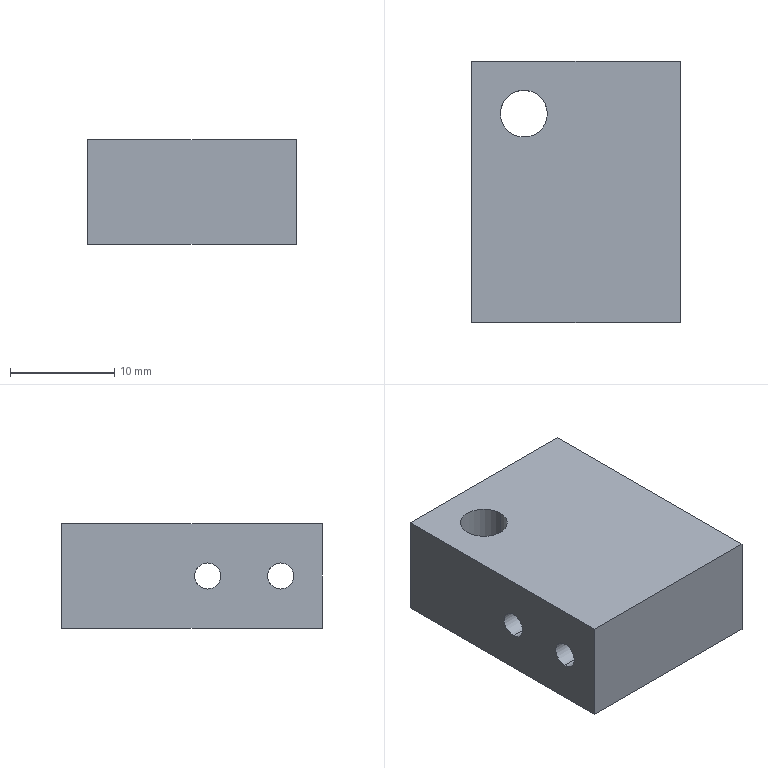Part | STEP file | 10-27 air distribution block | 1 solid | 19 faces | box 20 x 25 x 10 mm | volume 4387 mm3 | cylinder 10 | plane 6 | cone 3 | commonest cylinder face diameters 2.5 x6 4.2 x2 4.5 x2
STEP:
#1=CARTESIAN_POINT('',(0.3125,-1.5,3.75));
#2=VERTEX_POINT('',#1);
#3=CARTESIAN_POINT('',(0.3125,-1.5,6.25));
#4=VERTEX_POINT('',#3);
#5=CARTESIAN_POINT('',(0.3125,-1.5,3.75));
#6=CARTESIAN_POINT('',(0.3125,-1.415,3.75));
#7=CARTESIAN_POINT('',(0.3061,-1.332,3.759));
#8=CARTESIAN_POINT('',(0.2824,-1.17,3.792));
#9=CARTESIAN_POINT('',(0.2649,-1.09,3.816));
#10=CARTESIAN_POINT('',(0.2029,-0.8652,3.911));
#11=CARTESIAN_POINT('',(0.148,-0.7304,4.002));
#12=CARTESIAN_POINT('',(0.04358,-0.505,4.227));
#13=CARTESIAN_POINT('',(-0.006727,-0.4127,4.362));
#14=CARTESIAN_POINT('',(-0.06054,-0.3172,4.588));
#15=CARTESIAN_POINT('',(-0.07523,-0.292,4.668));
#16=CARTESIAN_POINT('',(-0.09477,-0.2587,4.831));
#17=CARTESIAN_POINT('',(-0.09991,-0.2502,4.914));
#18=CARTESIAN_POINT('',(-0.1002,-0.2497,5.166));
#19=CARTESIAN_POINT('',(-0.07907,-0.2843,5.334));
#20=CARTESIAN_POINT('',(-0.007079,-0.412,5.637));
#21=CARTESIAN_POINT('',(0.04343,-0.5047,5.773));
#22=CARTESIAN_POINT('',(0.1479,-0.7302,5.998));
#23=CARTESIAN_POINT('',(0.2027,-0.865,6.089));
#24=CARTESIAN_POINT('',(0.2646,-1.089,6.183));
#25=CARTESIAN_POINT('',(0.2822,-1.169,6.208));
#26=CARTESIAN_POINT('',(0.3061,-1.332,6.241));
#27=CARTESIAN_POINT('',(0.3125,-1.415,6.25));
#28=CARTESIAN_POINT('',(0.3125,-1.5,6.25));
#29=B_SPLINE_CURVE_WITH_KNOTS('',3,(#5,#6,#7,#8,#9,#10,#11,#12,#13,#14,#15,#16,#17,#18,#19,#20,#21,#22,#23,#24,#25,#26,#27,#28),.UNSPECIFIED.,.F.,.F.,(4,2,2,2,2,2,2,2,2,2,2,4),(0.,0.0002504,0.0005009,0.001002,0.001503,0.001753,0.002003,0.002504,0.003005,0.003506,0.003756,0.004007),.UNSPECIFIED.);
#30=EDGE_CURVE('',#2,#4,#29,.T.);
#31=ORIENTED_EDGE('',*,*,#30,.F.);
#32=CARTESIAN_POINT('',(0.3125,-1.5,6.25));
#33=CARTESIAN_POINT('',(0.3125,-1.67,6.25));
#34=CARTESIAN_POINT('',(0.2855,-1.836,6.215));
#35=CARTESIAN_POINT('',(0.2027,-2.135,6.089));
#36=CARTESIAN_POINT('',(0.1479,-2.27,5.998));
#37=CARTESIAN_POINT('',(0.04322,-2.496,5.772));
#38=CARTESIAN_POINT('',(-0.006762,-2.587,5.638));
#39=CARTESIAN_POINT('',(-0.06081,-2.683,5.411));
#40=CARTESIAN_POINT('',(-0.07535,-2.708,5.331));
#41=CARTESIAN_POINT('',(-0.09479,-2.741,5.169));
#42=CARTESIAN_POINT('',(-0.09996,-2.75,5.086));
#43=CARTESIAN_POINT('',(-0.1,-2.75,4.916));
#44=CARTESIAN_POINT('',(-0.09495,-2.742,4.833));
#45=CARTESIAN_POINT('',(-0.07549,-2.708,4.67));
#46=CARTESIAN_POINT('',(-0.06088,-2.683,4.589));
#47=CARTESIAN_POINT('',(-0.006947,-2.588,4.363));
#48=CARTESIAN_POINT('',(0.04358,-2.495,4.227));
#49=CARTESIAN_POINT('',(0.1483,-2.269,4.002));
#50=CARTESIAN_POINT('',(0.2028,-2.135,3.911));
#51=CARTESIAN_POINT('',(0.2649,-1.91,3.816));
#52=CARTESIAN_POINT('',(0.2825,-1.83,3.792));
#53=CARTESIAN_POINT('',(0.3061,-1.668,3.759));
#54=CARTESIAN_POINT('',(0.3125,-1.585,3.75));
#55=CARTESIAN_POINT('',(0.3125,-1.5,3.75));
#56=B_SPLINE_CURVE_WITH_KNOTS('',3,(#32,#33,#34,#35,#36,#37,#38,#39,#40,#41,#42,#43,#44,#45,#46,#47,#48,#49,#50,#51,#52,#53,#54,#55),.UNSPECIFIED.,.F.,.F.,(4,2,2,2,2,2,2,2,2,2,2,4),(0.004007,0.004507,0.005007,0.005507,0.005757,0.006007,0.006256,0.006506,0.007006,0.007506,0.007756,0.008006),.UNSPECIFIED.);
#57=EDGE_CURVE('',#4,#2,#56,.T.);
#58=ORIENTED_EDGE('',*,*,#57,.F.);
#59=EDGE_LOOP('',(#31,#58));
#60=FACE_BOUND('',#59,.T.);
#61=CARTESIAN_POINT('',(2.,-7.5,2.9));
#62=VERTEX_POINT('',#61);
#63=CARTESIAN_POINT('',(0.0385,-7.5,4.25));
#64=VERTEX_POINT('',#63);
#65=CARTESIAN_POINT('',(2.,-7.5,5.));
#66=DIRECTION('',(0.,1.,0.));
#67=DIRECTION('',(0.,0.,1.));
#68=AXIS2_PLACEMENT_3D('',#65,#66,#67);
#69=CIRCLE('',#68,2.1);
#70=EDGE_CURVE('',#62,#64,#69,.T.);
#71=ORIENTED_EDGE('',*,*,#70,.F.);
#72=CARTESIAN_POINT('',(2.,12.5,2.9));
#73=VERTEX_POINT('',#72);
#74=CARTESIAN_POINT('',(2.,12.5,2.9));
#75=DIRECTION('',(0.,1.,0.));
#76=VECTOR('',#75,1000.);
#77=LINE('',#74,#76);
#78=EDGE_CURVE('',#62,#73,#77,.T.);
#79=ORIENTED_EDGE('',*,*,#78,.T.);
#80=CARTESIAN_POINT('',(2.,12.5,7.1));
#81=VERTEX_POINT('',#80);
#82=CARTESIAN_POINT('',(2.,12.5,5.));
#83=DIRECTION('',(0.,1.,0.));
#84=DIRECTION('',(0.,0.,1.));
#85=AXIS2_PLACEMENT_3D('',#82,#83,#84);
#86=CIRCLE('',#85,2.1);
#87=EDGE_CURVE('',#73,#81,#86,.T.);
#88=ORIENTED_EDGE('',*,*,#87,.T.);
#89=CARTESIAN_POINT('',(2.,-7.5,7.1));
#90=VERTEX_POINT('',#89);
#91=CARTESIAN_POINT('',(2.,12.5,7.1));
#92=DIRECTION('',(0.,1.,0.));
#93=VECTOR('',#92,1000.);
#94=LINE('',#91,#93);
#95=EDGE_CURVE('',#90,#81,#94,.T.);
#96=ORIENTED_EDGE('',*,*,#95,.F.);
#97=CARTESIAN_POINT('',(0.0385,-7.5,5.75));
#98=VERTEX_POINT('',#97);
#99=CARTESIAN_POINT('',(2.,-7.5,5.));
#100=DIRECTION('',(0.,1.,0.));
#101=DIRECTION('',(0.,0.,1.));
#102=AXIS2_PLACEMENT_3D('',#99,#100,#101);
#103=CIRCLE('',#102,2.1);
#104=EDGE_CURVE('',#98,#90,#103,.T.);
#105=ORIENTED_EDGE('',*,*,#104,.F.);
#106=CARTESIAN_POINT('',(0.0385,-7.5,4.25));
#107=CARTESIAN_POINT('',(-0.001759,-7.421,4.355));
#108=CARTESIAN_POINT('',(-0.03659,-7.359,4.471));
#109=CARTESIAN_POINT('',(-0.0864,-7.272,4.728));
#110=CARTESIAN_POINT('',(-0.09994,-7.25,4.861));
#111=CARTESIAN_POINT('',(-0.1001,-7.25,5.275));
#112=CARTESIAN_POINT('',(-0.04206,-7.342,5.539));
#113=CARTESIAN_POINT('',(0.0385,-7.5,5.75));
#114=B_SPLINE_CURVE_WITH_KNOTS('',3,(#106,#107,#108,#109,#110,#111,#112,#113),.UNSPECIFIED.,.F.,.F.,(4,2,2,4),(0.,0.0004077,0.0008154,0.001631),.UNSPECIFIED.);
#115=EDGE_CURVE('',#64,#98,#114,.T.);
#116=ORIENTED_EDGE('',*,*,#115,.F.);
#117=EDGE_LOOP('',(#71,#79,#88,#96,#105,#116));
#118=FACE_OUTER_BOUND('',#117,.T.);
#119=CARTESIAN_POINT('',(2.,12.5,5.));
#120=DIRECTION('',(0.,1.,0.));
#121=DIRECTION('',(0.,0.,1.));
#122=AXIS2_PLACEMENT_3D('',#119,#120,#121);
#123=CYLINDRICAL_SURFACE('',#122,2.1);
#124=ADVANCED_FACE('',(#60,#118),#123,.F.);
#125=CARTESIAN_POINT('',(2.,-8.059,6.17));
#126=VERTEX_POINT('',#125);
#127=CARTESIAN_POINT('',(3.962,-7.5,5.75));
#128=VERTEX_POINT('',#127);
#129=CARTESIAN_POINT('',(2.,-8.059,6.17));
#130=CARTESIAN_POINT('',(2.176,-8.059,6.17));
#131=CARTESIAN_POINT('',(2.354,-8.038,6.162));
#132=CARTESIAN_POINT('',(2.697,-7.969,6.132));
#133=CARTESIAN_POINT('',(2.865,-7.921,6.11));
#134=CARTESIAN_POINT('',(3.195,-7.811,6.045));
#135=CARTESIAN_POINT('',(3.355,-7.751,6.004));
#136=CARTESIAN_POINT('',(3.666,-7.627,5.898));
#137=CARTESIAN_POINT('',(3.818,-7.563,5.833));
#138=CARTESIAN_POINT('',(3.962,-7.5,5.75));
#139=B_SPLINE_CURVE_WITH_KNOTS('',3,(#129,#130,#131,#132,#133,#134,#135,#136,#137,#138),.UNSPECIFIED.,.F.,.F.,(4,2,2,2,4),(0.002488,0.003016,0.003543,0.00407,0.004597),.UNSPECIFIED.);
#140=EDGE_CURVE('',#126,#128,#139,.T.);
#141=ORIENTED_EDGE('',*,*,#140,.F.);
#142=CARTESIAN_POINT('',(2.,-7.5,7.1));
#143=DIRECTION('',(0.,0.515,0.8572));
#144=VECTOR('',#143,1000.);
#145=LINE('',#142,#144);
#146=EDGE_CURVE('',#126,#90,#145,.T.);
#147=ORIENTED_EDGE('',*,*,#146,.T.);
#148=CARTESIAN_POINT('',(2.,-7.5,5.));
#149=DIRECTION('',(0.,1.,0.));
#150=DIRECTION('',(0.,0.,1.));
#151=AXIS2_PLACEMENT_3D('',#148,#149,#150);
#152=CIRCLE('',#151,2.1);
#153=EDGE_CURVE('',#90,#128,#152,.T.);
#154=ORIENTED_EDGE('',*,*,#153,.T.);
#155=EDGE_LOOP('',(#141,#147,#154));
#156=FACE_OUTER_BOUND('',#155,.T.);
#157=CARTESIAN_POINT('',(2.,-7.5,5.));
#158=DIRECTION('',(0.,1.,0.));
#159=DIRECTION('',(0.,0.,1.));
#160=AXIS2_PLACEMENT_3D('',#157,#158,#159);
#161=CONICAL_SURFACE('',#160,2.1,1.03);
#162=ADVANCED_FACE('',(#156),#161,.F.);
#163=CARTESIAN_POINT('',(-10.,-8.5,6.25));
#164=VERTEX_POINT('',#163);
#165=CARTESIAN_POINT('',(-10.,-8.5,3.75));
#166=VERTEX_POINT('',#165);
#167=CARTESIAN_POINT('',(-10.,-8.5,5.));
#168=DIRECTION('',(1.,0.,0.));
#169=DIRECTION('',(0.,0.,-1.));
#170=AXIS2_PLACEMENT_3D('',#167,#168,#169);
#171=CIRCLE('',#170,1.25);
#172=EDGE_CURVE('',#164,#166,#171,.T.);
#173=ORIENTED_EDGE('',*,*,#172,.F.);
#174=CARTESIAN_POINT('',(10.,-8.5,6.25));
#175=VERTEX_POINT('',#174);
#176=CARTESIAN_POINT('',(10.,-8.5,6.25));
#177=DIRECTION('',(1.,0.,0.));
#178=VECTOR('',#177,1000.);
#179=LINE('',#176,#178);
#180=EDGE_CURVE('',#164,#175,#179,.T.);
#181=ORIENTED_EDGE('',*,*,#180,.T.);
#182=CARTESIAN_POINT('',(10.,-8.5,3.75));
#183=VERTEX_POINT('',#182);
#184=CARTESIAN_POINT('',(10.,-8.5,5.));
#185=DIRECTION('',(1.,0.,0.));
#186=DIRECTION('',(0.,0.,-1.));
#187=AXIS2_PLACEMENT_3D('',#184,#185,#186);
#188=CIRCLE('',#187,1.25);
#189=EDGE_CURVE('',#175,#183,#188,.T.);
#190=ORIENTED_EDGE('',*,*,#189,.T.);
#191=CARTESIAN_POINT('',(10.,-8.5,3.75));
#192=DIRECTION('',(1.,0.,0.));
#193=VECTOR('',#192,1000.);
#194=LINE('',#191,#193);
#195=EDGE_CURVE('',#166,#183,#194,.T.);
#196=ORIENTED_EDGE('',*,*,#195,.F.);
#197=EDGE_LOOP('',(#173,#181,#190,#196));
#198=FACE_OUTER_BOUND('',#197,.T.);
#199=CARTESIAN_POINT('',(10.,-8.5,5.));
#200=DIRECTION('',(1.,0.,0.));
#201=DIRECTION('',(0.,0.,-1.));
#202=AXIS2_PLACEMENT_3D('',#199,#200,#201);
#203=CYLINDRICAL_SURFACE('',#202,1.25);
#204=ADVANCED_FACE('',(#198),#203,.F.);
#205=CARTESIAN_POINT('',(3.687,-1.5,3.75));
#206=VERTEX_POINT('',#205);
#207=CARTESIAN_POINT('',(3.687,-1.5,6.25));
#208=VERTEX_POINT('',#207);
#209=CARTESIAN_POINT('',(3.687,-1.5,3.75));
#210=CARTESIAN_POINT('',(3.687,-1.585,3.75));
#211=CARTESIAN_POINT('',(3.694,-1.668,3.759));
#212=CARTESIAN_POINT('',(3.718,-1.83,3.792));
#213=CARTESIAN_POINT('',(3.735,-1.91,3.816));
#214=CARTESIAN_POINT('',(3.797,-2.135,3.911));
#215=CARTESIAN_POINT('',(3.852,-2.27,4.002));
#216=CARTESIAN_POINT('',(3.956,-2.495,4.227));
#217=CARTESIAN_POINT('',(4.007,-2.587,4.362));
#218=CARTESIAN_POINT('',(4.061,-2.683,4.588));
#219=CARTESIAN_POINT('',(4.075,-2.708,4.668));
#220=CARTESIAN_POINT('',(4.095,-2.741,4.831));
#221=CARTESIAN_POINT('',(4.1,-2.75,4.914));
#222=CARTESIAN_POINT('',(4.1,-2.75,5.166));
#223=CARTESIAN_POINT('',(4.079,-2.716,5.334));
#224=CARTESIAN_POINT('',(4.007,-2.588,5.637));
#225=CARTESIAN_POINT('',(3.957,-2.495,5.773));
#226=CARTESIAN_POINT('',(3.852,-2.27,5.998));
#227=CARTESIAN_POINT('',(3.797,-2.135,6.089));
#228=CARTESIAN_POINT('',(3.735,-1.911,6.183));
#229=CARTESIAN_POINT('',(3.718,-1.831,6.208));
#230=CARTESIAN_POINT('',(3.694,-1.668,6.241));
#231=CARTESIAN_POINT('',(3.687,-1.585,6.25));
#232=CARTESIAN_POINT('',(3.687,-1.5,6.25));
#233=B_SPLINE_CURVE_WITH_KNOTS('',3,(#209,#210,#211,#212,#213,#214,#215,#216,#217,#218,#219,#220,#221,#222,#223,#224,#225,#226,#227,#228,#229,#230,#231,#232),.UNSPECIFIED.,.F.,.F.,(4,2,2,2,2,2,2,2,2,2,2,4),(0.,0.0002504,0.0005009,0.001002,0.001503,0.001753,0.002003,0.002504,0.003005,0.003506,0.003756,0.004007),.UNSPECIFIED.);
#234=EDGE_CURVE('',#206,#208,#233,.T.);
#235=ORIENTED_EDGE('',*,*,#234,.T.);
#236=CARTESIAN_POINT('',(10.,-1.5,6.25));
#237=VERTEX_POINT('',#236);
#238=CARTESIAN_POINT('',(10.,-1.5,6.25));
#239=DIRECTION('',(1.,0.,0.));
#240=VECTOR('',#239,1000.);
#241=LINE('',#238,#240);
#242=EDGE_CURVE('',#208,#237,#241,.T.);
#243=ORIENTED_EDGE('',*,*,#242,.T.);
#244=CARTESIAN_POINT('',(10.,-1.5,3.75));
#245=VERTEX_POINT('',#244);
#246=CARTESIAN_POINT('',(10.,-1.5,5.));
#247=DIRECTION('',(1.,0.,0.));
#248=DIRECTION('',(0.,0.,-1.));
#249=AXIS2_PLACEMENT_3D('',#246,#247,#248);
#250=CIRCLE('',#249,1.25);
#251=EDGE_CURVE('',#237,#245,#250,.T.);
#252=ORIENTED_EDGE('',*,*,#251,.T.);
#253=CARTESIAN_POINT('',(10.,-1.5,3.75));
#254=DIRECTION('',(1.,0.,0.));
#255=VECTOR('',#254,1000.);
#256=LINE('',#253,#255);
#257=EDGE_CURVE('',#206,#245,#256,.T.);
#258=ORIENTED_EDGE('',*,*,#257,.F.);
#259=EDGE_LOOP('',(#235,#243,#252,#258));
#260=FACE_OUTER_BOUND('',#259,.T.);
#261=CARTESIAN_POINT('',(10.,-1.5,5.));
#262=DIRECTION('',(1.,0.,0.));
#263=DIRECTION('',(0.,0.,-1.));
#264=AXIS2_PLACEMENT_3D('',#261,#262,#263);
#265=CYLINDRICAL_SURFACE('',#264,1.25);
#266=ADVANCED_FACE('',(#260),#265,.F.);
#267=CARTESIAN_POINT('',(-7.25,7.5,0.));
#268=VERTEX_POINT('',#267);
#269=CARTESIAN_POINT('',(-2.75,7.5,0.));
#270=VERTEX_POINT('',#269);
#271=CARTESIAN_POINT('',(-5.,7.5,0.));
#272=DIRECTION('',(0.,0.,1.));
#273=DIRECTION('',(1.,0.,0.));
#274=AXIS2_PLACEMENT_3D('',#271,#272,#273);
#275=CIRCLE('',#274,2.25);
#276=EDGE_CURVE('',#268,#270,#275,.T.);
#277=ORIENTED_EDGE('',*,*,#276,.F.);
#278=CARTESIAN_POINT('',(-7.25,7.5,10.));
#279=VERTEX_POINT('',#278);
#280=CARTESIAN_POINT('',(-7.25,7.5,0.));
#281=DIRECTION('',(0.,0.,1.));
#282=VECTOR('',#281,1000.);
#283=LINE('',#280,#282);
#284=EDGE_CURVE('',#268,#279,#283,.T.);
#285=ORIENTED_EDGE('',*,*,#284,.T.);
#286=CARTESIAN_POINT('',(-2.75,7.5,10.));
#287=VERTEX_POINT('',#286);
#288=CARTESIAN_POINT('',(-5.,7.5,10.));
#289=DIRECTION('',(0.,0.,1.));
#290=DIRECTION('',(1.,0.,0.));
#291=AXIS2_PLACEMENT_3D('',#288,#289,#290);
#292=CIRCLE('',#291,2.25);
#293=EDGE_CURVE('',#279,#287,#292,.T.);
#294=ORIENTED_EDGE('',*,*,#293,.T.);
#295=CARTESIAN_POINT('',(-2.75,7.5,0.));
#296=DIRECTION('',(0.,0.,1.));
#297=VECTOR('',#296,1000.);
#298=LINE('',#295,#297);
#299=EDGE_CURVE('',#270,#287,#298,.T.);
#300=ORIENTED_EDGE('',*,*,#299,.F.);
#301=EDGE_LOOP('',(#277,#285,#294,#300));
#302=FACE_OUTER_BOUND('',#301,.T.);
#303=CARTESIAN_POINT('',(-5.,7.5,0.));
#304=DIRECTION('',(0.,0.,1.));
#305=DIRECTION('',(1.,0.,0.));
#306=AXIS2_PLACEMENT_3D('',#303,#304,#305);
#307=CYLINDRICAL_SURFACE('',#306,2.25);
#308=ADVANCED_FACE('',(#302),#307,.F.);
#309=CARTESIAN_POINT('',(-10.,-1.5,6.25));
#310=VERTEX_POINT('',#309);
#311=CARTESIAN_POINT('',(-10.,-1.5,3.75));
#312=VERTEX_POINT('',#311);
#313=CARTESIAN_POINT('',(-10.,-1.5,5.));
#314=DIRECTION('',(1.,0.,0.));
#315=DIRECTION('',(0.,0.,-1.));
#316=AXIS2_PLACEMENT_3D('',#313,#314,#315);
#317=CIRCLE('',#316,1.25);
#318=EDGE_CURVE('',#310,#312,#317,.T.);
#319=ORIENTED_EDGE('',*,*,#318,.F.);
#320=CARTESIAN_POINT('',(10.,-1.5,6.25));
#321=DIRECTION('',(1.,0.,0.));
#322=VECTOR('',#321,1000.);
#323=LINE('',#320,#322);
#324=EDGE_CURVE('',#310,#4,#323,.T.);
#325=ORIENTED_EDGE('',*,*,#324,.T.);
#326=ORIENTED_EDGE('',*,*,#57,.T.);
#327=CARTESIAN_POINT('',(10.,-1.5,3.75));
#328=DIRECTION('',(1.,0.,0.));
#329=VECTOR('',#328,1000.);
#330=LINE('',#327,#329);
#331=EDGE_CURVE('',#312,#2,#330,.T.);
#332=ORIENTED_EDGE('',*,*,#331,.F.);
#333=EDGE_LOOP('',(#319,#325,#326,#332));
#334=FACE_OUTER_BOUND('',#333,.T.);
#335=CARTESIAN_POINT('',(10.,-1.5,5.));
#336=DIRECTION('',(1.,0.,0.));
#337=DIRECTION('',(0.,0.,-1.));
#338=AXIS2_PLACEMENT_3D('',#335,#336,#337);
#339=CYLINDRICAL_SURFACE('',#338,1.25);
#340=ADVANCED_FACE('',(#334),#339,.F.);
#341=ORIENTED_EDGE('',*,*,#324,.F.);
#342=CARTESIAN_POINT('',(-10.,-1.5,5.));
#343=DIRECTION('',(1.,0.,0.));
#344=DIRECTION('',(0.,0.,-1.));
#345=AXIS2_PLACEMENT_3D('',#342,#343,#344);
#346=CIRCLE('',#345,1.25);
#347=EDGE_CURVE('',#312,#310,#346,.T.);
#348=ORIENTED_EDGE('',*,*,#347,.F.);
#349=ORIENTED_EDGE('',*,*,#331,.T.);
#350=ORIENTED_EDGE('',*,*,#30,.T.);
#351=EDGE_LOOP('',(#341,#348,#349,#350));
#352=FACE_OUTER_BOUND('',#351,.T.);
#353=CARTESIAN_POINT('',(10.,-1.5,5.));
#354=DIRECTION('',(1.,0.,0.));
#355=DIRECTION('',(0.,0.,-1.));
#356=AXIS2_PLACEMENT_3D('',#353,#354,#355);
#357=CYLINDRICAL_SURFACE('',#356,1.25);
#358=ADVANCED_FACE('',(#352),#357,.F.);
#359=CARTESIAN_POINT('',(10.,-8.5,5.));
#360=DIRECTION('',(1.,0.,0.));
#361=DIRECTION('',(0.,0.,-1.));
#362=AXIS2_PLACEMENT_3D('',#359,#360,#361);
#363=CIRCLE('',#362,1.25);
#364=EDGE_CURVE('',#183,#175,#363,.T.);
#365=ORIENTED_EDGE('',*,*,#364,.F.);
#366=ORIENTED_EDGE('',*,*,#189,.F.);
#367=EDGE_LOOP('',(#365,#366));
#368=FACE_BOUND('',#367,.T.);
#369=CARTESIAN_POINT('',(10.,-1.5,5.));
#370=DIRECTION('',(1.,0.,0.));
#371=DIRECTION('',(0.,0.,-1.));
#372=AXIS2_PLACEMENT_3D('',#369,#370,#371);
#373=CIRCLE('',#372,1.25);
#374=EDGE_CURVE('',#245,#237,#373,.T.);
#375=ORIENTED_EDGE('',*,*,#374,.F.);
#376=ORIENTED_EDGE('',*,*,#251,.F.);
#377=EDGE_LOOP('',(#375,#376));
#378=FACE_BOUND('',#377,.T.);
#379=CARTESIAN_POINT('',(10.,-12.5,0.));
#380=VERTEX_POINT('',#379);
#381=CARTESIAN_POINT('',(10.,12.5,0.));
#382=VERTEX_POINT('',#381);
#383=CARTESIAN_POINT('',(10.,12.5,0.));
#384=DIRECTION('',(0.,1.,0.));
#385=VECTOR('',#384,1000.);
#386=LINE('',#383,#385);
#387=EDGE_CURVE('',#380,#382,#386,.T.);
#388=ORIENTED_EDGE('',*,*,#387,.T.);
#389=CARTESIAN_POINT('',(10.,12.5,10.));
#390=VERTEX_POINT('',#389);
#391=CARTESIAN_POINT('',(10.,12.5,10.));
#392=DIRECTION('',(0.,0.,-1.));
#393=VECTOR('',#392,1000.);
#394=LINE('',#391,#393);
#395=EDGE_CURVE('',#390,#382,#394,.T.);
#396=ORIENTED_EDGE('',*,*,#395,.F.);
#397=CARTESIAN_POINT('',(10.,-12.5,10.));
#398=VERTEX_POINT('',#397);
#399=CARTESIAN_POINT('',(10.,12.5,10.));
#400=DIRECTION('',(0.,1.,0.));
#401=VECTOR('',#400,1000.);
#402=LINE('',#399,#401);
#403=EDGE_CURVE('',#398,#390,#402,.T.);
#404=ORIENTED_EDGE('',*,*,#403,.F.);
#405=CARTESIAN_POINT('',(10.,-12.5,10.));
#406=DIRECTION('',(0.,0.,-1.));
#407=VECTOR('',#406,1000.);
#408=LINE('',#405,#407);
#409=EDGE_CURVE('',#398,#380,#408,.T.);
#410=ORIENTED_EDGE('',*,*,#409,.T.);
#411=EDGE_LOOP('',(#388,#396,#404,#410));
#412=FACE_OUTER_BOUND('',#411,.T.);
#413=CARTESIAN_POINT('',(10.,12.5,10.));
#414=DIRECTION('',(-1.,0.,0.));
#415=DIRECTION('',(0.,-1.,0.));
#416=AXIS2_PLACEMENT_3D('',#413,#414,#415);
#417=PLANE('',#416);
#418=ADVANCED_FACE('',(#368,#378,#412),#417,.F.);
#419=CARTESIAN_POINT('',(2.,12.5,5.));
#420=DIRECTION('',(0.,1.,0.));
#421=DIRECTION('',(0.,0.,1.));
#422=AXIS2_PLACEMENT_3D('',#419,#420,#421);
#423=CIRCLE('',#422,2.1);
#424=EDGE_CURVE('',#81,#73,#423,.T.);
#425=ORIENTED_EDGE('',*,*,#424,.F.);
#426=ORIENTED_EDGE('',*,*,#87,.F.);
#427=EDGE_LOOP('',(#425,#426));
#428=FACE_BOUND('',#427,.T.);
#429=CARTESIAN_POINT('',(-10.,12.5,0.));
#430=VERTEX_POINT('',#429);
#431=CARTESIAN_POINT('',(-10.,12.5,0.));
#432=DIRECTION('',(-1.,0.,0.));
#433=VECTOR('',#432,1000.);
#434=LINE('',#431,#433);
#435=EDGE_CURVE('',#382,#430,#434,.T.);
#436=ORIENTED_EDGE('',*,*,#435,.T.);
#437=CARTESIAN_POINT('',(-10.,12.5,10.));
#438=VERTEX_POINT('',#437);
#439=CARTESIAN_POINT('',(-10.,12.5,10.));
#440=DIRECTION('',(0.,0.,-1.));
#441=VECTOR('',#440,1000.);
#442=LINE('',#439,#441);
#443=EDGE_CURVE('',#438,#430,#442,.T.);
#444=ORIENTED_EDGE('',*,*,#443,.F.);
#445=CARTESIAN_POINT('',(-10.,12.5,10.));
#446=DIRECTION('',(-1.,0.,0.));
#447=VECTOR('',#446,1000.);
#448=LINE('',#445,#447);
#449=EDGE_CURVE('',#390,#438,#448,.T.);
#450=ORIENTED_EDGE('',*,*,#449,.F.);
#451=ORIENTED_EDGE('',*,*,#395,.T.);
#452=EDGE_LOOP('',(#436,#444,#450,#451));
#453=FACE_OUTER_BOUND('',#452,.T.);
#454=CARTESIAN_POINT('',(-10.,12.5,10.));
#455=DIRECTION('',(0.,-1.,0.));
#456=DIRECTION('',(0.,0.,-1.));
#457=AXIS2_PLACEMENT_3D('',#454,#455,#456);
#458=PLANE('',#457);
#459=ADVANCED_FACE('',(#428,#453),#458,.F.);
#460=CARTESIAN_POINT('',(-10.,-8.5,5.));
#461=DIRECTION('',(1.,0.,0.));
#462=DIRECTION('',(0.,0.,-1.));
#463=AXIS2_PLACEMENT_3D('',#460,#461,#462);
#464=CIRCLE('',#463,1.25);
#465=EDGE_CURVE('',#166,#164,#464,.T.);
#466=ORIENTED_EDGE('',*,*,#465,.T.);
#467=ORIENTED_EDGE('',*,*,#172,.T.);
#468=EDGE_LOOP('',(#466,#467));
#469=FACE_BOUND('',#468,.T.);
#470=ORIENTED_EDGE('',*,*,#347,.T.);
#471=ORIENTED_EDGE('',*,*,#318,.T.);
#472=EDGE_LOOP('',(#470,#471));
#473=FACE_BOUND('',#472,.T.);
#474=CARTESIAN_POINT('',(-10.,-12.5,0.));
#475=VERTEX_POINT('',#474);
#476=CARTESIAN_POINT('',(-10.,12.5,0.));
#477=DIRECTION('',(0.,-1.,0.));
#478=VECTOR('',#477,1000.);
#479=LINE('',#476,#478);
#480=EDGE_CURVE('',#430,#475,#479,.T.);
#481=ORIENTED_EDGE('',*,*,#480,.T.);
#482=CARTESIAN_POINT('',(-10.,-12.5,10.));
#483=VERTEX_POINT('',#482);
#484=CARTESIAN_POINT('',(-10.,-12.5,10.));
#485=DIRECTION('',(0.,0.,-1.));
#486=VECTOR('',#485,1000.);
#487=LINE('',#484,#486);
#488=EDGE_CURVE('',#483,#475,#487,.T.);
#489=ORIENTED_EDGE('',*,*,#488,.F.);
#490=CARTESIAN_POINT('',(-10.,12.5,10.));
#491=DIRECTION('',(0.,-1.,0.));
#492=VECTOR('',#491,1000.);
#493=LINE('',#490,#492);
#494=EDGE_CURVE('',#438,#483,#493,.T.);
#495=ORIENTED_EDGE('',*,*,#494,.F.);
#496=ORIENTED_EDGE('',*,*,#443,.T.);
#497=EDGE_LOOP('',(#481,#489,#495,#496));
#498=FACE_OUTER_BOUND('',#497,.T.);
#499=CARTESIAN_POINT('',(-10.,12.5,10.));
#500=DIRECTION('',(1.,0.,0.));
#501=DIRECTION('',(0.,1.,0.));
#502=AXIS2_PLACEMENT_3D('',#499,#500,#501);
#503=PLANE('',#502);
#504=ADVANCED_FACE('',(#469,#473,#498),#503,.F.);
#505=CARTESIAN_POINT('',(-10.,-12.5,0.));
#506=DIRECTION('',(1.,0.,0.));
#507=VECTOR('',#506,1000.);
#508=LINE('',#505,#507);
#509=EDGE_CURVE('',#475,#380,#508,.T.);
#510=ORIENTED_EDGE('',*,*,#509,.T.);
#511=ORIENTED_EDGE('',*,*,#409,.F.);
#512=CARTESIAN_POINT('',(-10.,-12.5,10.));
#513=DIRECTION('',(1.,0.,0.));
#514=VECTOR('',#513,1000.);
#515=LINE('',#512,#514);
#516=EDGE_CURVE('',#483,#398,#515,.T.);
#517=ORIENTED_EDGE('',*,*,#516,.F.);
#518=ORIENTED_EDGE('',*,*,#488,.T.);
#519=EDGE_LOOP('',(#510,#511,#517,#518));
#520=FACE_OUTER_BOUND('',#519,.T.);
#521=CARTESIAN_POINT('',(-10.,-12.5,10.));
#522=DIRECTION('',(0.,1.,0.));
#523=DIRECTION('',(0.,0.,1.));
#524=AXIS2_PLACEMENT_3D('',#521,#522,#523);
#525=PLANE('',#524);
#526=ADVANCED_FACE('',(#520),#525,.F.);
#527=CARTESIAN_POINT('',(-5.,7.5,10.));
#528=DIRECTION('',(0.,0.,1.));
#529=DIRECTION('',(1.,0.,0.));
#530=AXIS2_PLACEMENT_3D('',#527,#528,#529);
#531=CIRCLE('',#530,2.25);
#532=EDGE_CURVE('',#287,#279,#531,.T.);
#533=ORIENTED_EDGE('',*,*,#532,.F.);
#534=ORIENTED_EDGE('',*,*,#293,.F.);
#535=EDGE_LOOP('',(#533,#534));
#536=FACE_BOUND('',#535,.T.);
#537=ORIENTED_EDGE('',*,*,#403,.T.);
#538=ORIENTED_EDGE('',*,*,#449,.T.);
#539=ORIENTED_EDGE('',*,*,#494,.T.);
#540=ORIENTED_EDGE('',*,*,#516,.T.);
#541=EDGE_LOOP('',(#537,#538,#539,#540));
#542=FACE_OUTER_BOUND('',#541,.T.);
#543=CARTESIAN_POINT('',(10.,-12.5,10.));
#544=DIRECTION('',(0.,0.,1.));
#545=DIRECTION('',(1.,0.,0.));
#546=AXIS2_PLACEMENT_3D('',#543,#544,#545);
#547=PLANE('',#546);
#548=ADVANCED_FACE('',(#536,#542),#547,.T.);
#549=CARTESIAN_POINT('',(-5.,7.5,0.));
#550=DIRECTION('',(0.,0.,1.));
#551=DIRECTION('',(1.,0.,0.));
#552=AXIS2_PLACEMENT_3D('',#549,#550,#551);
#553=CIRCLE('',#552,2.25);
#554=EDGE_CURVE('',#270,#268,#553,.T.);
#555=ORIENTED_EDGE('',*,*,#554,.T.);
#556=ORIENTED_EDGE('',*,*,#276,.T.);
#557=EDGE_LOOP('',(#555,#556));
#558=FACE_BOUND('',#557,.T.);
#559=ORIENTED_EDGE('',*,*,#387,.F.);
#560=ORIENTED_EDGE('',*,*,#509,.F.);
#561=ORIENTED_EDGE('',*,*,#480,.F.);
#562=ORIENTED_EDGE('',*,*,#435,.F.);
#563=EDGE_LOOP('',(#559,#560,#561,#562));
#564=FACE_OUTER_BOUND('',#563,.T.);
#565=CARTESIAN_POINT('',(10.,-12.5,0.));
#566=DIRECTION('',(0.,0.,1.));
#567=DIRECTION('',(1.,0.,0.));
#568=AXIS2_PLACEMENT_3D('',#565,#566,#567);
#569=PLANE('',#568);
#570=ADVANCED_FACE('',(#558,#564),#569,.F.);
#571=ORIENTED_EDGE('',*,*,#284,.F.);
#572=ORIENTED_EDGE('',*,*,#554,.F.);
#573=ORIENTED_EDGE('',*,*,#299,.T.);
#574=ORIENTED_EDGE('',*,*,#532,.T.);
#575=EDGE_LOOP('',(#571,#572,#573,#574));
#576=FACE_OUTER_BOUND('',#575,.T.);
#577=CARTESIAN_POINT('',(-5.,7.5,0.));
#578=DIRECTION('',(0.,0.,1.));
#579=DIRECTION('',(1.,0.,0.));
#580=AXIS2_PLACEMENT_3D('',#577,#578,#579);
#581=CYLINDRICAL_SURFACE('',#580,2.25);
#582=ADVANCED_FACE('',(#576),#581,.F.);
#583=ORIENTED_EDGE('',*,*,#242,.F.);
#584=CARTESIAN_POINT('',(3.687,-1.5,6.25));
#585=CARTESIAN_POINT('',(3.687,-1.33,6.25));
#586=CARTESIAN_POINT('',(3.714,-1.164,6.215));
#587=CARTESIAN_POINT('',(3.797,-0.8647,6.089));
#588=CARTESIAN_POINT('',(3.852,-0.7301,5.998));
#589=CARTESIAN_POINT('',(3.957,-0.5043,5.772));
#590=CARTESIAN_POINT('',(4.007,-0.4126,5.638));
#591=CARTESIAN_POINT('',(4.061,-0.3167,5.411));
#592=CARTESIAN_POINT('',(4.075,-0.2918,5.331));
#593=CARTESIAN_POINT('',(4.095,-0.2587,5.169));
#594=CARTESIAN_POINT('',(4.1,-0.2501,5.086));
#595=CARTESIAN_POINT('',(4.1,-0.2499,4.916));
#596=CARTESIAN_POINT('',(4.095,-0.2584,4.833));
#597=CARTESIAN_POINT('',(4.075,-0.2916,4.67));
#598=CARTESIAN_POINT('',(4.061,-0.3166,4.589));
#599=CARTESIAN_POINT('',(4.007,-0.4123,4.363));
#600=CARTESIAN_POINT('',(3.956,-0.505,4.227));
#601=CARTESIAN_POINT('',(3.852,-0.7309,4.002));
#602=CARTESIAN_POINT('',(3.797,-0.8651,3.911));
#603=CARTESIAN_POINT('',(3.735,-1.09,3.816));
#604=CARTESIAN_POINT('',(3.718,-1.17,3.792));
#605=CARTESIAN_POINT('',(3.694,-1.332,3.759));
#606=CARTESIAN_POINT('',(3.687,-1.415,3.75));
#607=CARTESIAN_POINT('',(3.687,-1.5,3.75));
#608=B_SPLINE_CURVE_WITH_KNOTS('',3,(#584,#585,#586,#587,#588,#589,#590,#591,#592,#593,#594,#595,#596,#597,#598,#599,#600,#601,#602,#603,#604,#605,#606,#607),.UNSPECIFIED.,.F.,.F.,(4,2,2,2,2,2,2,2,2,2,2,4),(0.004007,0.004507,0.005007,0.005507,0.005757,0.006007,0.006256,0.006506,0.007006,0.007506,0.007756,0.008006),.UNSPECIFIED.);
#609=EDGE_CURVE('',#208,#206,#608,.T.);
#610=ORIENTED_EDGE('',*,*,#609,.T.);
#611=ORIENTED_EDGE('',*,*,#257,.T.);
#612=ORIENTED_EDGE('',*,*,#374,.T.);
#613=EDGE_LOOP('',(#583,#610,#611,#612));
#614=FACE_OUTER_BOUND('',#613,.T.);
#615=CARTESIAN_POINT('',(10.,-1.5,5.));
#616=DIRECTION('',(1.,0.,0.));
#617=DIRECTION('',(0.,0.,-1.));
#618=AXIS2_PLACEMENT_3D('',#615,#616,#617);
#619=CYLINDRICAL_SURFACE('',#618,1.25);
#620=ADVANCED_FACE('',(#614),#619,.F.);
#621=ORIENTED_EDGE('',*,*,#180,.F.);
#622=ORIENTED_EDGE('',*,*,#465,.F.);
#623=ORIENTED_EDGE('',*,*,#195,.T.);
#624=ORIENTED_EDGE('',*,*,#364,.T.);
#625=EDGE_LOOP('',(#621,#622,#623,#624));
#626=FACE_OUTER_BOUND('',#625,.T.);
#627=CARTESIAN_POINT('',(3.962,-7.5,4.25));
#628=VERTEX_POINT('',#627);
#629=CARTESIAN_POINT('',(3.962,-7.5,5.75));
#630=CARTESIAN_POINT('',(4.002,-7.421,5.645));
#631=CARTESIAN_POINT('',(4.037,-7.359,5.529));
#632=CARTESIAN_POINT('',(4.086,-7.272,5.272));
#633=CARTESIAN_POINT('',(4.1,-7.25,5.139));
#634=CARTESIAN_POINT('',(4.1,-7.25,4.725));
#635=CARTESIAN_POINT('',(4.042,-7.342,4.461));
#636=CARTESIAN_POINT('',(3.962,-7.5,4.25));
#637=B_SPLINE_CURVE_WITH_KNOTS('',3,(#629,#630,#631,#632,#633,#634,#635,#636),.UNSPECIFIED.,.F.,.F.,(4,2,2,4),(0.,0.0004077,0.0008154,0.001631),.UNSPECIFIED.);
#638=EDGE_CURVE('',#128,#628,#637,.T.);
#639=ORIENTED_EDGE('',*,*,#638,.T.);
#640=CARTESIAN_POINT('',(3.962,-7.5,4.25));
#641=CARTESIAN_POINT('',(3.819,-7.562,4.167));
#642=CARTESIAN_POINT('',(3.666,-7.627,4.101));
#643=CARTESIAN_POINT('',(3.354,-7.752,3.996));
#644=CARTESIAN_POINT('',(3.195,-7.812,3.955));
#645=CARTESIAN_POINT('',(2.867,-7.92,3.891));
#646=CARTESIAN_POINT('',(2.698,-7.969,3.868));
#647=CARTESIAN_POINT('',(2.353,-8.038,3.838));
#648=CARTESIAN_POINT('',(2.179,-8.059,3.83));
#649=CARTESIAN_POINT('',(1.827,-8.059,3.83));
#650=CARTESIAN_POINT('',(1.649,-8.039,3.838));
#651=CARTESIAN_POINT('',(1.305,-7.97,3.868));
#652=CARTESIAN_POINT('',(1.137,-7.921,3.89));
#653=CARTESIAN_POINT('',(0.8058,-7.812,3.954));
#654=CARTESIAN_POINT('',(0.6455,-7.751,3.996));
#655=CARTESIAN_POINT('',(0.3342,-7.627,4.101));
#656=CARTESIAN_POINT('',(0.1821,-7.563,4.166));
#657=CARTESIAN_POINT('',(0.0385,-7.5,4.25));
#658=B_SPLINE_CURVE_WITH_KNOTS('',3,(#640,#641,#642,#643,#644,#645,#646,#647,#648,#649,#650,#651,#652,#653,#654,#655,#656,#657),.UNSPECIFIED.,.F.,.F.,(4,2,2,2,2,2,2,2,4),(0.0003736,0.0009015,0.001429,0.001957,0.002485,0.003013,0.003541,0.004069,0.004597),.UNSPECIFIED.);
#659=EDGE_CURVE('',#628,#64,#658,.T.);
#660=ORIENTED_EDGE('',*,*,#659,.T.);
#661=ORIENTED_EDGE('',*,*,#115,.T.);
#662=CARTESIAN_POINT('',(0.0385,-7.5,5.75));
#663=CARTESIAN_POINT('',(0.1811,-7.562,5.833));
#664=CARTESIAN_POINT('',(0.3346,-7.627,5.899));
#665=CARTESIAN_POINT('',(0.6466,-7.752,6.005));
#666=CARTESIAN_POINT('',(0.8064,-7.812,6.046));
#667=CARTESIAN_POINT('',(1.135,-7.921,6.109));
#668=CARTESIAN_POINT('',(1.305,-7.969,6.132));
#669=CARTESIAN_POINT('',(1.65,-8.039,6.162));
#670=CARTESIAN_POINT('',(1.824,-8.059,6.17));
#671=CARTESIAN_POINT('',(2.,-8.059,6.17));
#672=B_SPLINE_CURVE_WITH_KNOTS('',3,(#662,#663,#664,#665,#666,#667,#668,#669,#670,#671),.UNSPECIFIED.,.F.,.F.,(4,2,2,2,4),(0.0003736,0.0009023,0.001431,0.00196,0.002488),.UNSPECIFIED.);
#673=EDGE_CURVE('',#98,#126,#672,.T.);
#674=ORIENTED_EDGE('',*,*,#673,.T.);
#675=ORIENTED_EDGE('',*,*,#140,.T.);
#676=EDGE_LOOP('',(#639,#660,#661,#674,#675));
#677=FACE_BOUND('',#676,.T.);
#678=CARTESIAN_POINT('',(10.,-8.5,5.));
#679=DIRECTION('',(1.,0.,0.));
#680=DIRECTION('',(0.,0.,-1.));
#681=AXIS2_PLACEMENT_3D('',#678,#679,#680);
#682=CYLINDRICAL_SURFACE('',#681,1.25);
#683=ADVANCED_FACE('',(#626,#677),#682,.F.);
#684=CARTESIAN_POINT('',(2.,-7.5,5.));
#685=DIRECTION('',(0.,1.,0.));
#686=DIRECTION('',(0.,0.,1.));
#687=AXIS2_PLACEMENT_3D('',#684,#685,#686);
#688=CIRCLE('',#687,2.1);
#689=EDGE_CURVE('',#628,#62,#688,.T.);
#690=ORIENTED_EDGE('',*,*,#689,.T.);
#691=ORIENTED_EDGE('',*,*,#70,.T.);
#692=ORIENTED_EDGE('',*,*,#659,.F.);
#693=EDGE_LOOP('',(#690,#691,#692));
#694=FACE_OUTER_BOUND('',#693,.T.);
#695=CARTESIAN_POINT('',(2.,-7.5,5.));
#696=DIRECTION('',(0.,1.,0.));
#697=DIRECTION('',(0.,0.,1.));
#698=AXIS2_PLACEMENT_3D('',#695,#696,#697);
#699=CONICAL_SURFACE('',#698,2.1,1.03);
#700=ADVANCED_FACE('',(#694),#699,.F.);
#701=ORIENTED_EDGE('',*,*,#146,.F.);
#702=ORIENTED_EDGE('',*,*,#673,.F.);
#703=ORIENTED_EDGE('',*,*,#104,.T.);
#704=EDGE_LOOP('',(#701,#702,#703));
#705=FACE_OUTER_BOUND('',#704,.T.);
#706=CARTESIAN_POINT('',(2.,-7.5,5.));
#707=DIRECTION('',(0.,1.,0.));
#708=DIRECTION('',(0.,0.,1.));
#709=AXIS2_PLACEMENT_3D('',#706,#707,#708);
#710=CONICAL_SURFACE('',#709,2.1,1.03);
#711=ADVANCED_FACE('',(#705),#710,.F.);
#712=ORIENTED_EDGE('',*,*,#78,.F.);
#713=ORIENTED_EDGE('',*,*,#689,.F.);
#714=ORIENTED_EDGE('',*,*,#638,.F.);
#715=ORIENTED_EDGE('',*,*,#153,.F.);
#716=ORIENTED_EDGE('',*,*,#95,.T.);
#717=ORIENTED_EDGE('',*,*,#424,.T.);
#718=EDGE_LOOP('',(#712,#713,#714,#715,#716,#717));
#719=FACE_OUTER_BOUND('',#718,.T.);
#720=ORIENTED_EDGE('',*,*,#234,.F.);
#721=ORIENTED_EDGE('',*,*,#609,.F.);
#722=EDGE_LOOP('',(#720,#721));
#723=FACE_BOUND('',#722,.T.);
#724=CARTESIAN_POINT('',(2.,12.5,5.));
#725=DIRECTION('',(0.,1.,0.));
#726=DIRECTION('',(0.,0.,1.));
#727=AXIS2_PLACEMENT_3D('',#724,#725,#726);
#728=CYLINDRICAL_SURFACE('',#727,2.1);
#729=ADVANCED_FACE('',(#719,#723),#728,.F.);
#730=CLOSED_SHELL('',(#124,#162,#204,#266,#308,#340,#358,#418,#459,#504,#526,#548,#570,#582,#620,#683,#700,#711,#729));
#731=MANIFOLD_SOLID_BREP('',#730);
#732=CARTESIAN_POINT('',(0.,0.,0.));
#733=DIRECTION('',(0.,0.,1.));
#734=DIRECTION('',(1.,0.,0.));
#735=AXIS2_PLACEMENT_3D('',#732,#733,#734);
#736=(LENGTH_UNIT()NAMED_UNIT(*)SI_UNIT(.MILLI.,.METRE.));
#737=UNCERTAINTY_MEASURE_WITH_UNIT(LENGTH_MEASURE(0.00001),#736,'','');
#738=(NAMED_UNIT(*)PLANE_ANGLE_UNIT()SI_UNIT($,.RADIAN.));
#739=(NAMED_UNIT(*)SI_UNIT($,.STERADIAN.)SOLID_ANGLE_UNIT());
#740=(GEOMETRIC_REPRESENTATION_CONTEXT(3)GLOBAL_UNCERTAINTY_ASSIGNED_CONTEXT((#737))GLOBAL_UNIT_ASSIGNED_CONTEXT((#736,#738,#739))REPRESENTATION_CONTEXT('',''));
#741=ADVANCED_BREP_SHAPE_REPRESENTATION('',(#731,#735),#740);